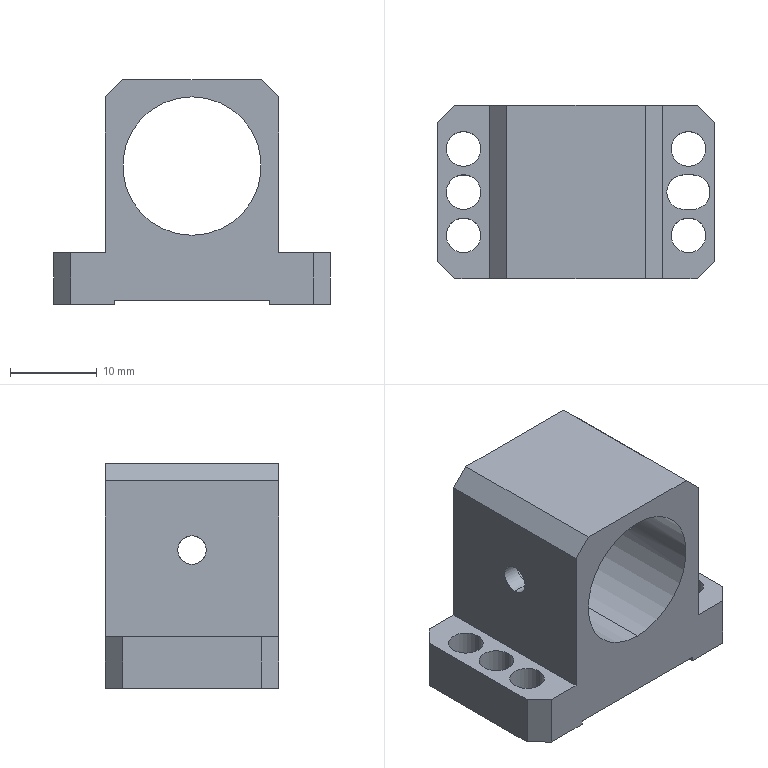Part | 1 solid | 41 faces | box 32 x 20 x 26 mm | volume 6999 mm3 | plane 22 | cylinder 19 | commonest cylinder face diameters 4 x13 3.3 x4 16 x2
STEP:
#1=CARTESIAN_POINT('',(-7.828,0.,-8.35));
#2=VERTEX_POINT('',#1);
#3=CARTESIAN_POINT('',(-7.828,0.,-11.65));
#4=VERTEX_POINT('',#3);
#5=CARTESIAN_POINT('',(-7.828,0.,-8.35));
#6=CARTESIAN_POINT('',(-7.828,-0.4372,-8.35));
#7=CARTESIAN_POINT('',(-7.915,-1.29,-8.708));
#8=CARTESIAN_POINT('',(-8.042,-1.83,-9.998));
#9=CARTESIAN_POINT('',(-7.915,-1.291,-11.293));
#10=CARTESIAN_POINT('',(-7.828,-0.4372,-11.65));
#11=CARTESIAN_POINT('',(-7.828,0.,-11.65));
#12=B_SPLINE_CURVE_WITH_KNOTS('',3,(#5,#6,#7,#8,#9,#10,#11),.UNSPECIFIED.,.F.,.F.,(4,1,1,1,4),(0.,0.001293,0.002586,0.003878,0.005171),.UNSPECIFIED.);
#13=EDGE_CURVE('',#2,#4,#12,.T.);
#14=ORIENTED_EDGE('',*,*,#13,.T.);
#15=CARTESIAN_POINT('',(-10.,0.,-11.65));
#16=VERTEX_POINT('',#15);
#17=CARTESIAN_POINT('',(-10.,0.,-11.65));
#18=DIRECTION('',(-1.,0.,0.));
#19=VECTOR('',#18,1000.);
#20=LINE('',#17,#19);
#21=EDGE_CURVE('',#4,#16,#20,.T.);
#22=ORIENTED_EDGE('',*,*,#21,.T.);
#23=CARTESIAN_POINT('',(-10.,0.,-8.35));
#24=VERTEX_POINT('',#23);
#25=CARTESIAN_POINT('',(-10.,0.,-10.));
#26=DIRECTION('',(-1.,0.,0.));
#27=DIRECTION('',(0.,0.,1.));
#28=AXIS2_PLACEMENT_3D('',#25,#26,#27);
#29=CIRCLE('',#28,1.65);
#30=EDGE_CURVE('',#16,#24,#29,.T.);
#31=ORIENTED_EDGE('',*,*,#30,.T.);
#32=CARTESIAN_POINT('',(-10.,0.,-8.35));
#33=DIRECTION('',(-1.,0.,0.));
#34=VECTOR('',#33,1000.);
#35=LINE('',#32,#34);
#36=EDGE_CURVE('',#2,#24,#35,.T.);
#37=ORIENTED_EDGE('',*,*,#36,.F.);
#38=EDGE_LOOP('',(#14,#22,#31,#37));
#39=FACE_BOUND('',#38,.T.);
#40=CARTESIAN_POINT('',(-10.,0.,-10.));
#41=DIRECTION('',(-1.,0.,0.));
#42=DIRECTION('',(0.,0.,-1.));
#43=AXIS2_PLACEMENT_3D('',#40,#41,#42);
#44=CYLINDRICAL_SURFACE('',#43,1.65);
#45=ADVANCED_FACE('',(#39),#44,.F.);
#46=CARTESIAN_POINT('',(7.828,0.,-11.65));
#47=VERTEX_POINT('',#46);
#48=CARTESIAN_POINT('',(7.828,0.,-8.35));
#49=VERTEX_POINT('',#48);
#50=CARTESIAN_POINT('',(7.828,0.,-11.65));
#51=CARTESIAN_POINT('',(7.828,-0.4372,-11.65));
#52=CARTESIAN_POINT('',(7.915,-1.29,-11.292));
#53=CARTESIAN_POINT('',(8.042,-1.83,-10.002));
#54=CARTESIAN_POINT('',(7.915,-1.291,-8.707));
#55=CARTESIAN_POINT('',(7.828,-0.4372,-8.35));
#56=CARTESIAN_POINT('',(7.828,0.,-8.35));
#57=B_SPLINE_CURVE_WITH_KNOTS('',3,(#50,#51,#52,#53,#54,#55,#56),.UNSPECIFIED.,.F.,.F.,(4,1,1,1,4),(0.,0.001293,0.002586,0.003878,0.005171),.UNSPECIFIED.);
#58=EDGE_CURVE('',#47,#49,#57,.T.);
#59=ORIENTED_EDGE('',*,*,#58,.T.);
#60=CARTESIAN_POINT('',(10.,0.,-8.35));
#61=VERTEX_POINT('',#60);
#62=CARTESIAN_POINT('',(10.,0.,-8.35));
#63=DIRECTION('',(1.,0.,0.));
#64=VECTOR('',#63,1000.);
#65=LINE('',#62,#64);
#66=EDGE_CURVE('',#49,#61,#65,.T.);
#67=ORIENTED_EDGE('',*,*,#66,.T.);
#68=CARTESIAN_POINT('',(10.,0.,-11.65));
#69=VERTEX_POINT('',#68);
#70=CARTESIAN_POINT('',(10.,0.,-10.));
#71=DIRECTION('',(1.,0.,0.));
#72=DIRECTION('',(0.,0.,-1.));
#73=AXIS2_PLACEMENT_3D('',#70,#71,#72);
#74=CIRCLE('',#73,1.65);
#75=EDGE_CURVE('',#61,#69,#74,.T.);
#76=ORIENTED_EDGE('',*,*,#75,.T.);
#77=CARTESIAN_POINT('',(10.,0.,-11.65));
#78=DIRECTION('',(1.,0.,0.));
#79=VECTOR('',#78,1000.);
#80=LINE('',#77,#79);
#81=EDGE_CURVE('',#47,#69,#80,.T.);
#82=ORIENTED_EDGE('',*,*,#81,.F.);
#83=EDGE_LOOP('',(#59,#67,#76,#82));
#84=FACE_BOUND('',#83,.T.);
#85=CARTESIAN_POINT('',(10.,0.,-10.));
#86=DIRECTION('',(1.,0.,0.));
#87=DIRECTION('',(0.,0.,1.));
#88=AXIS2_PLACEMENT_3D('',#85,#86,#87);
#89=CYLINDRICAL_SURFACE('',#88,1.65);
#90=ADVANCED_FACE('',(#84),#89,.F.);
#91=CARTESIAN_POINT('',(12.5,2.,-20.));
#92=VERTEX_POINT('',#91);
#93=CARTESIAN_POINT('',(10.5,0.,-20.));
#94=VERTEX_POINT('',#93);
#95=CARTESIAN_POINT('',(12.5,0.,-20.));
#96=DIRECTION('',(0.,0.,1.));
#97=DIRECTION('',(1.,0.,0.));
#98=AXIS2_PLACEMENT_3D('',#95,#96,#97);
#99=CIRCLE('',#98,2.);
#100=EDGE_CURVE('',#92,#94,#99,.T.);
#101=ORIENTED_EDGE('',*,*,#100,.T.);
#102=CARTESIAN_POINT('',(10.5,0.,-26.));
#103=VERTEX_POINT('',#102);
#104=CARTESIAN_POINT('',(10.5,0.,-16.));
#105=DIRECTION('',(0.,0.,-1.));
#106=VECTOR('',#105,1000.);
#107=LINE('',#104,#106);
#108=EDGE_CURVE('',#94,#103,#107,.T.);
#109=ORIENTED_EDGE('',*,*,#108,.T.);
#110=CARTESIAN_POINT('',(12.5,2.,-26.));
#111=VERTEX_POINT('',#110);
#112=CARTESIAN_POINT('',(12.5,0.,-26.));
#113=DIRECTION('',(0.,0.,-1.));
#114=DIRECTION('',(-1.,0.,0.));
#115=AXIS2_PLACEMENT_3D('',#112,#113,#114);
#116=CIRCLE('',#115,2.);
#117=EDGE_CURVE('',#103,#111,#116,.T.);
#118=ORIENTED_EDGE('',*,*,#117,.T.);
#119=CARTESIAN_POINT('',(12.5,2.,-16.));
#120=DIRECTION('',(0.,0.,-1.));
#121=VECTOR('',#120,1000.);
#122=LINE('',#119,#121);
#123=EDGE_CURVE('',#92,#111,#122,.T.);
#124=ORIENTED_EDGE('',*,*,#123,.F.);
#125=EDGE_LOOP('',(#101,#109,#118,#124));
#126=FACE_BOUND('',#125,.T.);
#127=CARTESIAN_POINT('',(12.5,0.,-16.));
#128=DIRECTION('',(0.,0.,-1.));
#129=DIRECTION('',(1.,0.,0.));
#130=AXIS2_PLACEMENT_3D('',#127,#128,#129);
#131=CYLINDRICAL_SURFACE('',#130,2.);
#132=ADVANCED_FACE('',(#126),#131,.F.);
#133=CARTESIAN_POINT('',(-15.,0.,-20.));
#134=VERTEX_POINT('',#133);
#135=CARTESIAN_POINT('',(-11.,0.,-20.));
#136=VERTEX_POINT('',#135);
#137=CARTESIAN_POINT('',(-13.,0.,-20.));
#138=DIRECTION('',(0.,0.,1.));
#139=DIRECTION('',(1.,0.,0.));
#140=AXIS2_PLACEMENT_3D('',#137,#138,#139);
#141=CIRCLE('',#140,2.);
#142=EDGE_CURVE('',#134,#136,#141,.T.);
#143=ORIENTED_EDGE('',*,*,#142,.T.);
#144=CARTESIAN_POINT('',(-11.,0.,-26.));
#145=VERTEX_POINT('',#144);
#146=CARTESIAN_POINT('',(-11.,0.,-16.));
#147=DIRECTION('',(0.,0.,-1.));
#148=VECTOR('',#147,1000.);
#149=LINE('',#146,#148);
#150=EDGE_CURVE('',#136,#145,#149,.T.);
#151=ORIENTED_EDGE('',*,*,#150,.T.);
#152=CARTESIAN_POINT('',(-15.,0.,-26.));
#153=VERTEX_POINT('',#152);
#154=CARTESIAN_POINT('',(-13.,0.,-26.));
#155=DIRECTION('',(0.,0.,-1.));
#156=DIRECTION('',(-1.,0.,0.));
#157=AXIS2_PLACEMENT_3D('',#154,#155,#156);
#158=CIRCLE('',#157,2.);
#159=EDGE_CURVE('',#145,#153,#158,.T.);
#160=ORIENTED_EDGE('',*,*,#159,.T.);
#161=CARTESIAN_POINT('',(-15.,0.,-16.));
#162=DIRECTION('',(0.,0.,-1.));
#163=VECTOR('',#162,1000.);
#164=LINE('',#161,#163);
#165=EDGE_CURVE('',#134,#153,#164,.T.);
#166=ORIENTED_EDGE('',*,*,#165,.F.);
#167=EDGE_LOOP('',(#143,#151,#160,#166));
#168=FACE_BOUND('',#167,.T.);
#169=CARTESIAN_POINT('',(-13.,0.,-16.));
#170=DIRECTION('',(0.,0.,-1.));
#171=DIRECTION('',(1.,0.,0.));
#172=AXIS2_PLACEMENT_3D('',#169,#170,#171);
#173=CYLINDRICAL_SURFACE('',#172,2.);
#174=ADVANCED_FACE('',(#168),#173,.F.);
#175=CARTESIAN_POINT('',(11.,-5.,-20.));
#176=VERTEX_POINT('',#175);
#177=CARTESIAN_POINT('',(15.,-5.,-20.));
#178=VERTEX_POINT('',#177);
#179=CARTESIAN_POINT('',(13.,-5.,-20.));
#180=DIRECTION('',(0.,0.,1.));
#181=DIRECTION('',(1.,0.,0.));
#182=AXIS2_PLACEMENT_3D('',#179,#180,#181);
#183=CIRCLE('',#182,2.);
#184=EDGE_CURVE('',#176,#178,#183,.T.);
#185=ORIENTED_EDGE('',*,*,#184,.T.);
#186=CARTESIAN_POINT('',(15.,-5.,-26.));
#187=VERTEX_POINT('',#186);
#188=CARTESIAN_POINT('',(15.,-5.,-6.));
#189=DIRECTION('',(0.,0.,-1.));
#190=VECTOR('',#189,1000.);
#191=LINE('',#188,#190);
#192=EDGE_CURVE('',#178,#187,#191,.T.);
#193=ORIENTED_EDGE('',*,*,#192,.T.);
#194=CARTESIAN_POINT('',(11.,-5.,-26.));
#195=VERTEX_POINT('',#194);
#196=CARTESIAN_POINT('',(13.,-5.,-26.));
#197=DIRECTION('',(0.,0.,-1.));
#198=DIRECTION('',(-1.,0.,0.));
#199=AXIS2_PLACEMENT_3D('',#196,#197,#198);
#200=CIRCLE('',#199,2.);
#201=EDGE_CURVE('',#187,#195,#200,.T.);
#202=ORIENTED_EDGE('',*,*,#201,.T.);
#203=CARTESIAN_POINT('',(11.,-5.,-6.));
#204=DIRECTION('',(0.,0.,-1.));
#205=VECTOR('',#204,1000.);
#206=LINE('',#203,#205);
#207=EDGE_CURVE('',#176,#195,#206,.T.);
#208=ORIENTED_EDGE('',*,*,#207,.F.);
#209=EDGE_LOOP('',(#185,#193,#202,#208));
#210=FACE_BOUND('',#209,.T.);
#211=CARTESIAN_POINT('',(13.,-5.,-6.));
#212=DIRECTION('',(0.,0.,-1.));
#213=DIRECTION('',(1.,0.,0.));
#214=AXIS2_PLACEMENT_3D('',#211,#212,#213);
#215=CYLINDRICAL_SURFACE('',#214,2.);
#216=ADVANCED_FACE('',(#210),#215,.F.);
#217=CARTESIAN_POINT('',(-15.,5.,-20.));
#218=VERTEX_POINT('',#217);
#219=CARTESIAN_POINT('',(-11.,5.,-20.));
#220=VERTEX_POINT('',#219);
#221=CARTESIAN_POINT('',(-13.,5.,-20.));
#222=DIRECTION('',(0.,0.,1.));
#223=DIRECTION('',(1.,0.,0.));
#224=AXIS2_PLACEMENT_3D('',#221,#222,#223);
#225=CIRCLE('',#224,2.);
#226=EDGE_CURVE('',#218,#220,#225,.T.);
#227=ORIENTED_EDGE('',*,*,#226,.T.);
#228=CARTESIAN_POINT('',(-11.,5.,-26.));
#229=VERTEX_POINT('',#228);
#230=CARTESIAN_POINT('',(-11.,5.,-6.));
#231=DIRECTION('',(0.,0.,-1.));
#232=VECTOR('',#231,1000.);
#233=LINE('',#230,#232);
#234=EDGE_CURVE('',#220,#229,#233,.T.);
#235=ORIENTED_EDGE('',*,*,#234,.T.);
#236=CARTESIAN_POINT('',(-15.,5.,-26.));
#237=VERTEX_POINT('',#236);
#238=CARTESIAN_POINT('',(-13.,5.,-26.));
#239=DIRECTION('',(0.,0.,-1.));
#240=DIRECTION('',(-1.,0.,0.));
#241=AXIS2_PLACEMENT_3D('',#238,#239,#240);
#242=CIRCLE('',#241,2.);
#243=EDGE_CURVE('',#229,#237,#242,.T.);
#244=ORIENTED_EDGE('',*,*,#243,.T.);
#245=CARTESIAN_POINT('',(-15.,5.,-6.));
#246=DIRECTION('',(0.,0.,-1.));
#247=VECTOR('',#246,1000.);
#248=LINE('',#245,#247);
#249=EDGE_CURVE('',#218,#237,#248,.T.);
#250=ORIENTED_EDGE('',*,*,#249,.F.);
#251=EDGE_LOOP('',(#227,#235,#244,#250));
#252=FACE_BOUND('',#251,.T.);
#253=CARTESIAN_POINT('',(-13.,5.,-6.));
#254=DIRECTION('',(0.,0.,-1.));
#255=DIRECTION('',(1.,0.,0.));
#256=AXIS2_PLACEMENT_3D('',#253,#254,#255);
#257=CYLINDRICAL_SURFACE('',#256,2.);
#258=ADVANCED_FACE('',(#252),#257,.F.);
#259=CARTESIAN_POINT('',(-15.,-5.,-20.));
#260=VERTEX_POINT('',#259);
#261=CARTESIAN_POINT('',(-11.,-5.,-20.));
#262=VERTEX_POINT('',#261);
#263=CARTESIAN_POINT('',(-13.,-5.,-20.));
#264=DIRECTION('',(0.,0.,1.));
#265=DIRECTION('',(1.,0.,0.));
#266=AXIS2_PLACEMENT_3D('',#263,#264,#265);
#267=CIRCLE('',#266,2.);
#268=EDGE_CURVE('',#260,#262,#267,.T.);
#269=ORIENTED_EDGE('',*,*,#268,.T.);
#270=CARTESIAN_POINT('',(-11.,-5.,-26.));
#271=VERTEX_POINT('',#270);
#272=CARTESIAN_POINT('',(-11.,-5.,-6.));
#273=DIRECTION('',(0.,0.,-1.));
#274=VECTOR('',#273,1000.);
#275=LINE('',#272,#274);
#276=EDGE_CURVE('',#262,#271,#275,.T.);
#277=ORIENTED_EDGE('',*,*,#276,.T.);
#278=CARTESIAN_POINT('',(-15.,-5.,-26.));
#279=VERTEX_POINT('',#278);
#280=CARTESIAN_POINT('',(-13.,-5.,-26.));
#281=DIRECTION('',(0.,0.,-1.));
#282=DIRECTION('',(-1.,0.,0.));
#283=AXIS2_PLACEMENT_3D('',#280,#281,#282);
#284=CIRCLE('',#283,2.);
#285=EDGE_CURVE('',#271,#279,#284,.T.);
#286=ORIENTED_EDGE('',*,*,#285,.T.);
#287=CARTESIAN_POINT('',(-15.,-5.,-6.));
#288=DIRECTION('',(0.,0.,-1.));
#289=VECTOR('',#288,1000.);
#290=LINE('',#287,#289);
#291=EDGE_CURVE('',#260,#279,#290,.T.);
#292=ORIENTED_EDGE('',*,*,#291,.F.);
#293=EDGE_LOOP('',(#269,#277,#286,#292));
#294=FACE_BOUND('',#293,.T.);
#295=CARTESIAN_POINT('',(-13.,-5.,-6.));
#296=DIRECTION('',(0.,0.,-1.));
#297=DIRECTION('',(1.,0.,0.));
#298=AXIS2_PLACEMENT_3D('',#295,#296,#297);
#299=CYLINDRICAL_SURFACE('',#298,2.);
#300=ADVANCED_FACE('',(#294),#299,.F.);
#301=CARTESIAN_POINT('',(11.,5.,-20.));
#302=VERTEX_POINT('',#301);
#303=CARTESIAN_POINT('',(15.,5.,-20.));
#304=VERTEX_POINT('',#303);
#305=CARTESIAN_POINT('',(13.,5.,-20.));
#306=DIRECTION('',(0.,0.,1.));
#307=DIRECTION('',(1.,0.,0.));
#308=AXIS2_PLACEMENT_3D('',#305,#306,#307);
#309=CIRCLE('',#308,2.);
#310=EDGE_CURVE('',#302,#304,#309,.T.);
#311=ORIENTED_EDGE('',*,*,#310,.T.);
#312=CARTESIAN_POINT('',(15.,5.,-26.));
#313=VERTEX_POINT('',#312);
#314=CARTESIAN_POINT('',(15.,5.,-6.));
#315=DIRECTION('',(0.,0.,-1.));
#316=VECTOR('',#315,1000.);
#317=LINE('',#314,#316);
#318=EDGE_CURVE('',#304,#313,#317,.T.);
#319=ORIENTED_EDGE('',*,*,#318,.T.);
#320=CARTESIAN_POINT('',(11.,5.,-26.));
#321=VERTEX_POINT('',#320);
#322=CARTESIAN_POINT('',(13.,5.,-26.));
#323=DIRECTION('',(0.,0.,-1.));
#324=DIRECTION('',(-1.,0.,0.));
#325=AXIS2_PLACEMENT_3D('',#322,#323,#324);
#326=CIRCLE('',#325,2.);
#327=EDGE_CURVE('',#313,#321,#326,.T.);
#328=ORIENTED_EDGE('',*,*,#327,.T.);
#329=CARTESIAN_POINT('',(11.,5.,-6.));
#330=DIRECTION('',(0.,0.,-1.));
#331=VECTOR('',#330,1000.);
#332=LINE('',#329,#331);
#333=EDGE_CURVE('',#302,#321,#332,.T.);
#334=ORIENTED_EDGE('',*,*,#333,.F.);
#335=EDGE_LOOP('',(#311,#319,#328,#334));
#336=FACE_BOUND('',#335,.T.);
#337=CARTESIAN_POINT('',(13.,5.,-6.));
#338=DIRECTION('',(0.,0.,-1.));
#339=DIRECTION('',(1.,0.,0.));
#340=AXIS2_PLACEMENT_3D('',#337,#338,#339);
#341=CYLINDRICAL_SURFACE('',#340,2.);
#342=ADVANCED_FACE('',(#336),#341,.F.);
#343=ORIENTED_EDGE('',*,*,#13,.F.);
#344=CARTESIAN_POINT('',(-7.828,0.,-11.65));
#345=CARTESIAN_POINT('',(-7.828,0.4372,-11.65));
#346=CARTESIAN_POINT('',(-7.915,1.29,-11.292));
#347=CARTESIAN_POINT('',(-8.042,1.83,-10.002));
#348=CARTESIAN_POINT('',(-7.915,1.291,-8.707));
#349=CARTESIAN_POINT('',(-7.828,0.4372,-8.35));
#350=CARTESIAN_POINT('',(-7.828,0.,-8.35));
#351=B_SPLINE_CURVE_WITH_KNOTS('',3,(#344,#345,#346,#347,#348,#349,#350),.UNSPECIFIED.,.F.,.F.,(4,1,1,1,4),(0.,0.001293,0.002586,0.003878,0.005171),.UNSPECIFIED.);
#352=EDGE_CURVE('',#4,#2,#351,.T.);
#353=ORIENTED_EDGE('',*,*,#352,.F.);
#354=EDGE_LOOP('',(#343,#353));
#355=FACE_BOUND('',#354,.T.);
#356=CARTESIAN_POINT('',(0.,10.,-18.));
#357=VERTEX_POINT('',#356);
#358=CARTESIAN_POINT('',(0.,10.,-2.));
#359=VERTEX_POINT('',#358);
#360=CARTESIAN_POINT('',(0.,10.,-10.));
#361=DIRECTION('',(0.,1.,0.));
#362=DIRECTION('',(0.,0.,1.));
#363=AXIS2_PLACEMENT_3D('',#360,#361,#362);
#364=CIRCLE('',#363,8.);
#365=EDGE_CURVE('',#357,#359,#364,.T.);
#366=ORIENTED_EDGE('',*,*,#365,.T.);
#367=CARTESIAN_POINT('',(0.,-10.,-2.));
#368=VERTEX_POINT('',#367);
#369=CARTESIAN_POINT('',(0.,10.,-2.));
#370=DIRECTION('',(0.,-1.,0.));
#371=VECTOR('',#370,1000.);
#372=LINE('',#369,#371);
#373=EDGE_CURVE('',#359,#368,#372,.T.);
#374=ORIENTED_EDGE('',*,*,#373,.T.);
#375=CARTESIAN_POINT('',(0.,-10.,-18.));
#376=VERTEX_POINT('',#375);
#377=CARTESIAN_POINT('',(0.,-10.,-10.));
#378=DIRECTION('',(0.,1.,0.));
#379=DIRECTION('',(0.,0.,1.));
#380=AXIS2_PLACEMENT_3D('',#377,#378,#379);
#381=CIRCLE('',#380,8.);
#382=EDGE_CURVE('',#376,#368,#381,.T.);
#383=ORIENTED_EDGE('',*,*,#382,.F.);
#384=CARTESIAN_POINT('',(0.,10.,-18.));
#385=DIRECTION('',(0.,-1.,0.));
#386=VECTOR('',#385,1000.);
#387=LINE('',#384,#386);
#388=EDGE_CURVE('',#357,#376,#387,.T.);
#389=ORIENTED_EDGE('',*,*,#388,.F.);
#390=EDGE_LOOP('',(#366,#374,#383,#389));
#391=FACE_BOUND('',#390,.T.);
#392=CARTESIAN_POINT('',(0.,10.,-10.));
#393=DIRECTION('',(0.,-1.,0.));
#394=DIRECTION('',(0.,0.,1.));
#395=AXIS2_PLACEMENT_3D('',#392,#393,#394);
#396=CYLINDRICAL_SURFACE('',#395,8.);
#397=ADVANCED_FACE('',(#355,#391),#396,.F.);
#398=CARTESIAN_POINT('',(13.,5.,-26.));
#399=DIRECTION('',(0.,0.,-1.));
#400=DIRECTION('',(-1.,0.,0.));
#401=AXIS2_PLACEMENT_3D('',#398,#399,#400);
#402=CIRCLE('',#401,2.);
#403=EDGE_CURVE('',#321,#313,#402,.T.);
#404=ORIENTED_EDGE('',*,*,#403,.F.);
#405=ORIENTED_EDGE('',*,*,#327,.F.);
#406=EDGE_LOOP('',(#404,#405));
#407=FACE_BOUND('',#406,.T.);
#408=CARTESIAN_POINT('',(13.,-5.,-26.));
#409=DIRECTION('',(0.,0.,-1.));
#410=DIRECTION('',(-1.,0.,0.));
#411=AXIS2_PLACEMENT_3D('',#408,#409,#410);
#412=CIRCLE('',#411,2.);
#413=EDGE_CURVE('',#195,#187,#412,.T.);
#414=ORIENTED_EDGE('',*,*,#413,.F.);
#415=ORIENTED_EDGE('',*,*,#201,.F.);
#416=EDGE_LOOP('',(#414,#415));
#417=FACE_BOUND('',#416,.T.);
#418=CARTESIAN_POINT('',(13.5,-2.,-26.));
#419=VERTEX_POINT('',#418);
#420=CARTESIAN_POINT('',(12.5,-2.,-26.));
#421=VERTEX_POINT('',#420);
#422=CARTESIAN_POINT('',(12.5,-2.,-26.));
#423=DIRECTION('',(-1.,0.,0.));
#424=VECTOR('',#423,1000.);
#425=LINE('',#422,#424);
#426=EDGE_CURVE('',#419,#421,#425,.T.);
#427=ORIENTED_EDGE('',*,*,#426,.F.);
#428=CARTESIAN_POINT('',(13.5,2.,-26.));
#429=VERTEX_POINT('',#428);
#430=CARTESIAN_POINT('',(13.5,0.,-26.));
#431=DIRECTION('',(0.,0.,-1.));
#432=DIRECTION('',(-1.,0.,0.));
#433=AXIS2_PLACEMENT_3D('',#430,#431,#432);
#434=CIRCLE('',#433,2.);
#435=EDGE_CURVE('',#429,#419,#434,.T.);
#436=ORIENTED_EDGE('',*,*,#435,.F.);
#437=CARTESIAN_POINT('',(12.5,2.,-26.));
#438=DIRECTION('',(1.,0.,0.));
#439=VECTOR('',#438,1000.);
#440=LINE('',#437,#439);
#441=EDGE_CURVE('',#111,#429,#440,.T.);
#442=ORIENTED_EDGE('',*,*,#441,.F.);
#443=ORIENTED_EDGE('',*,*,#117,.F.);
#444=CARTESIAN_POINT('',(12.5,0.,-26.));
#445=DIRECTION('',(0.,0.,-1.));
#446=DIRECTION('',(-1.,0.,0.));
#447=AXIS2_PLACEMENT_3D('',#444,#445,#446);
#448=CIRCLE('',#447,2.);
#449=EDGE_CURVE('',#421,#103,#448,.T.);
#450=ORIENTED_EDGE('',*,*,#449,.F.);
#451=EDGE_LOOP('',(#427,#436,#442,#443,#450));
#452=FACE_BOUND('',#451,.T.);
#453=CARTESIAN_POINT('',(14.,-10.,-26.));
#454=VERTEX_POINT('',#453);
#455=CARTESIAN_POINT('',(9.,-10.,-26.));
#456=VERTEX_POINT('',#455);
#457=CARTESIAN_POINT('',(10.,-10.,-26.));
#458=DIRECTION('',(-1.,0.,0.));
#459=VECTOR('',#458,1000.);
#460=LINE('',#457,#459);
#461=EDGE_CURVE('',#454,#456,#460,.T.);
#462=ORIENTED_EDGE('',*,*,#461,.T.);
#463=CARTESIAN_POINT('',(9.,10.,-26.));
#464=VERTEX_POINT('',#463);
#465=CARTESIAN_POINT('',(9.,10.,-26.));
#466=DIRECTION('',(0.,-1.,0.));
#467=VECTOR('',#466,1000.);
#468=LINE('',#465,#467);
#469=EDGE_CURVE('',#464,#456,#468,.T.);
#470=ORIENTED_EDGE('',*,*,#469,.F.);
#471=CARTESIAN_POINT('',(14.,10.,-26.));
#472=VERTEX_POINT('',#471);
#473=CARTESIAN_POINT('',(10.,10.,-26.));
#474=DIRECTION('',(-1.,0.,0.));
#475=VECTOR('',#474,1000.);
#476=LINE('',#473,#475);
#477=EDGE_CURVE('',#472,#464,#476,.T.);
#478=ORIENTED_EDGE('',*,*,#477,.F.);
#479=CARTESIAN_POINT('',(16.,8.,-26.));
#480=VERTEX_POINT('',#479);
#481=CARTESIAN_POINT('',(16.,8.,-26.));
#482=DIRECTION('',(0.7071,-0.7071,0.));
#483=VECTOR('',#482,1000.);
#484=LINE('',#481,#483);
#485=EDGE_CURVE('',#472,#480,#484,.T.);
#486=ORIENTED_EDGE('',*,*,#485,.T.);
#487=CARTESIAN_POINT('',(16.,-8.,-26.));
#488=VERTEX_POINT('',#487);
#489=CARTESIAN_POINT('',(16.,10.,-26.));
#490=DIRECTION('',(0.,-1.,0.));
#491=VECTOR('',#490,1000.);
#492=LINE('',#489,#491);
#493=EDGE_CURVE('',#480,#488,#492,.T.);
#494=ORIENTED_EDGE('',*,*,#493,.T.);
#495=CARTESIAN_POINT('',(14.,-10.,-26.));
#496=DIRECTION('',(-0.7071,-0.7071,0.));
#497=VECTOR('',#496,1000.);
#498=LINE('',#495,#497);
#499=EDGE_CURVE('',#488,#454,#498,.T.);
#500=ORIENTED_EDGE('',*,*,#499,.T.);
#501=EDGE_LOOP('',(#462,#470,#478,#486,#494,#500));
#502=FACE_BOUND('',#501,.T.);
#503=CARTESIAN_POINT('',(10.,10.,-26.));
#504=DIRECTION('',(0.,0.,1.));
#505=DIRECTION('',(-1.,0.,0.));
#506=AXIS2_PLACEMENT_3D('',#503,#504,#505);
#507=PLANE('',#506);
#508=ADVANCED_FACE('',(#407,#417,#452,#502),#507,.F.);
#509=CARTESIAN_POINT('',(9.,10.,-25.5));
#510=VERTEX_POINT('',#509);
#511=CARTESIAN_POINT('',(9.,10.,-25.5));
#512=DIRECTION('',(0.,0.,-1.));
#513=VECTOR('',#512,1000.);
#514=LINE('',#511,#513);
#515=EDGE_CURVE('',#510,#464,#514,.T.);
#516=ORIENTED_EDGE('',*,*,#515,.F.);
#517=CARTESIAN_POINT('',(-9.,10.,-25.5));
#518=VERTEX_POINT('',#517);
#519=CARTESIAN_POINT('',(9.,10.,-25.5));
#520=DIRECTION('',(1.,0.,0.));
#521=VECTOR('',#520,1000.);
#522=LINE('',#519,#521);
#523=EDGE_CURVE('',#518,#510,#522,.T.);
#524=ORIENTED_EDGE('',*,*,#523,.F.);
#525=CARTESIAN_POINT('',(-9.,10.,-26.));
#526=VERTEX_POINT('',#525);
#527=CARTESIAN_POINT('',(-9.,10.,-25.5));
#528=DIRECTION('',(0.,0.,-1.));
#529=VECTOR('',#528,1000.);
#530=LINE('',#527,#529);
#531=EDGE_CURVE('',#518,#526,#530,.T.);
#532=ORIENTED_EDGE('',*,*,#531,.T.);
#533=CARTESIAN_POINT('',(-14.,10.,-26.));
#534=VERTEX_POINT('',#533);
#535=CARTESIAN_POINT('',(10.,10.,-26.));
#536=DIRECTION('',(-1.,0.,0.));
#537=VECTOR('',#536,1000.);
#538=LINE('',#535,#537);
#539=EDGE_CURVE('',#526,#534,#538,.T.);
#540=ORIENTED_EDGE('',*,*,#539,.T.);
#541=CARTESIAN_POINT('',(-14.,10.,-20.));
#542=VERTEX_POINT('',#541);
#543=CARTESIAN_POINT('',(-14.,10.,-13.));
#544=DIRECTION('',(0.,0.,1.));
#545=VECTOR('',#544,1000.);
#546=LINE('',#543,#545);
#547=EDGE_CURVE('',#534,#542,#546,.T.);
#548=ORIENTED_EDGE('',*,*,#547,.T.);
#549=CARTESIAN_POINT('',(-10.,10.,-20.));
#550=VERTEX_POINT('',#549);
#551=CARTESIAN_POINT('',(-16.,10.,-20.));
#552=DIRECTION('',(-1.,0.,0.));
#553=VECTOR('',#552,1000.);
#554=LINE('',#551,#553);
#555=EDGE_CURVE('',#550,#542,#554,.T.);
#556=ORIENTED_EDGE('',*,*,#555,.F.);
#557=CARTESIAN_POINT('',(-10.,10.,-2.));
#558=VERTEX_POINT('',#557);
#559=CARTESIAN_POINT('',(-10.,10.,0.));
#560=DIRECTION('',(0.,0.,1.));
#561=VECTOR('',#560,1000.);
#562=LINE('',#559,#561);
#563=EDGE_CURVE('',#550,#558,#562,.T.);
#564=ORIENTED_EDGE('',*,*,#563,.T.);
#565=CARTESIAN_POINT('',(-8.,10.,0.));
#566=VERTEX_POINT('',#565);
#567=CARTESIAN_POINT('',(-10.5,10.,-2.5));
#568=DIRECTION('',(0.7071,0.,0.7071));
#569=VECTOR('',#568,1000.);
#570=LINE('',#567,#569);
#571=EDGE_CURVE('',#558,#566,#570,.T.);
#572=ORIENTED_EDGE('',*,*,#571,.T.);
#573=CARTESIAN_POINT('',(8.,10.,0.));
#574=VERTEX_POINT('',#573);
#575=CARTESIAN_POINT('',(10.,10.,0.));
#576=DIRECTION('',(1.,0.,0.));
#577=VECTOR('',#576,1000.);
#578=LINE('',#575,#577);
#579=EDGE_CURVE('',#566,#574,#578,.T.);
#580=ORIENTED_EDGE('',*,*,#579,.T.);
#581=CARTESIAN_POINT('',(10.,10.,-2.));
#582=VERTEX_POINT('',#581);
#583=CARTESIAN_POINT('',(10.5,10.,-2.5));
#584=DIRECTION('',(0.7071,0.,-0.7071));
#585=VECTOR('',#584,1000.);
#586=LINE('',#583,#585);
#587=EDGE_CURVE('',#574,#582,#586,.T.);
#588=ORIENTED_EDGE('',*,*,#587,.T.);
#589=CARTESIAN_POINT('',(10.,10.,-20.));
#590=VERTEX_POINT('',#589);
#591=CARTESIAN_POINT('',(10.,10.,0.));
#592=DIRECTION('',(0.,0.,-1.));
#593=VECTOR('',#592,1000.);
#594=LINE('',#591,#593);
#595=EDGE_CURVE('',#582,#590,#594,.T.);
#596=ORIENTED_EDGE('',*,*,#595,.T.);
#597=CARTESIAN_POINT('',(14.,10.,-20.));
#598=VERTEX_POINT('',#597);
#599=CARTESIAN_POINT('',(-16.,10.,-20.));
#600=DIRECTION('',(-1.,0.,0.));
#601=VECTOR('',#600,1000.);
#602=LINE('',#599,#601);
#603=EDGE_CURVE('',#598,#590,#602,.T.);
#604=ORIENTED_EDGE('',*,*,#603,.F.);
#605=CARTESIAN_POINT('',(14.,10.,-13.));
#606=DIRECTION('',(0.,0.,-1.));
#607=VECTOR('',#606,1000.);
#608=LINE('',#605,#607);
#609=EDGE_CURVE('',#598,#472,#608,.T.);
#610=ORIENTED_EDGE('',*,*,#609,.T.);
#611=ORIENTED_EDGE('',*,*,#477,.T.);
#612=EDGE_LOOP('',(#516,#524,#532,#540,#548,#556,#564,#572,#580,#588,#596,#604,#610,#611));
#613=FACE_BOUND('',#612,.T.);
#614=ORIENTED_EDGE('',*,*,#365,.F.);
#615=CARTESIAN_POINT('',(0.,10.,-10.));
#616=DIRECTION('',(0.,1.,0.));
#617=DIRECTION('',(0.,0.,1.));
#618=AXIS2_PLACEMENT_3D('',#615,#616,#617);
#619=CIRCLE('',#618,8.);
#620=EDGE_CURVE('',#359,#357,#619,.T.);
#621=ORIENTED_EDGE('',*,*,#620,.F.);
#622=EDGE_LOOP('',(#614,#621));
#623=FACE_BOUND('',#622,.T.);
#624=CARTESIAN_POINT('',(0.,10.,-13.));
#625=DIRECTION('',(0.,1.,0.));
#626=DIRECTION('',(0.,0.,-1.));
#627=AXIS2_PLACEMENT_3D('',#624,#625,#626);
#628=PLANE('',#627);
#629=ADVANCED_FACE('',(#613,#623),#628,.T.);
#630=CARTESIAN_POINT('',(9.,-10.,-25.5));
#631=VERTEX_POINT('',#630);
#632=CARTESIAN_POINT('',(-9.,-10.,-25.5));
#633=VERTEX_POINT('',#632);
#634=CARTESIAN_POINT('',(9.,-10.,-25.5));
#635=DIRECTION('',(-1.,0.,0.));
#636=VECTOR('',#635,1000.);
#637=LINE('',#634,#636);
#638=EDGE_CURVE('',#631,#633,#637,.T.);
#639=ORIENTED_EDGE('',*,*,#638,.F.);
#640=CARTESIAN_POINT('',(9.,-10.,-25.5));
#641=DIRECTION('',(0.,0.,-1.));
#642=VECTOR('',#641,1000.);
#643=LINE('',#640,#642);
#644=EDGE_CURVE('',#631,#456,#643,.T.);
#645=ORIENTED_EDGE('',*,*,#644,.T.);
#646=ORIENTED_EDGE('',*,*,#461,.F.);
#647=CARTESIAN_POINT('',(14.,-10.,-20.));
#648=VERTEX_POINT('',#647);
#649=CARTESIAN_POINT('',(14.,-10.,-20.));
#650=DIRECTION('',(0.,0.,1.));
#651=VECTOR('',#650,1000.);
#652=LINE('',#649,#651);
#653=EDGE_CURVE('',#454,#648,#652,.T.);
#654=ORIENTED_EDGE('',*,*,#653,.T.);
#655=CARTESIAN_POINT('',(10.,-10.,-20.));
#656=VERTEX_POINT('',#655);
#657=CARTESIAN_POINT('',(-16.,-10.,-20.));
#658=DIRECTION('',(-1.,0.,0.));
#659=VECTOR('',#658,1000.);
#660=LINE('',#657,#659);
#661=EDGE_CURVE('',#648,#656,#660,.T.);
#662=ORIENTED_EDGE('',*,*,#661,.T.);
#663=CARTESIAN_POINT('',(10.,-10.,-2.));
#664=VERTEX_POINT('',#663);
#665=CARTESIAN_POINT('',(10.,-10.,0.));
#666=DIRECTION('',(0.,0.,-1.));
#667=VECTOR('',#666,1000.);
#668=LINE('',#665,#667);
#669=EDGE_CURVE('',#664,#656,#668,.T.);
#670=ORIENTED_EDGE('',*,*,#669,.F.);
#671=CARTESIAN_POINT('',(8.,-10.,0.));
#672=VERTEX_POINT('',#671);
#673=CARTESIAN_POINT('',(10.,-10.,-2.));
#674=DIRECTION('',(-0.7071,0.,0.7071));
#675=VECTOR('',#674,1000.);
#676=LINE('',#673,#675);
#677=EDGE_CURVE('',#664,#672,#676,.T.);
#678=ORIENTED_EDGE('',*,*,#677,.T.);
#679=CARTESIAN_POINT('',(-8.,-10.,0.));
#680=VERTEX_POINT('',#679);
#681=CARTESIAN_POINT('',(10.,-10.,0.));
#682=DIRECTION('',(1.,0.,0.));
#683=VECTOR('',#682,1000.);
#684=LINE('',#681,#683);
#685=EDGE_CURVE('',#680,#672,#684,.T.);
#686=ORIENTED_EDGE('',*,*,#685,.F.);
#687=CARTESIAN_POINT('',(-10.,-10.,-2.));
#688=VERTEX_POINT('',#687);
#689=CARTESIAN_POINT('',(-8.,-10.,0.));
#690=DIRECTION('',(-0.7071,0.,-0.7071));
#691=VECTOR('',#690,1000.);
#692=LINE('',#689,#691);
#693=EDGE_CURVE('',#680,#688,#692,.T.);
#694=ORIENTED_EDGE('',*,*,#693,.T.);
#695=CARTESIAN_POINT('',(-10.,-10.,-20.));
#696=VERTEX_POINT('',#695);
#697=CARTESIAN_POINT('',(-10.,-10.,0.));
#698=DIRECTION('',(0.,0.,1.));
#699=VECTOR('',#698,1000.);
#700=LINE('',#697,#699);
#701=EDGE_CURVE('',#696,#688,#700,.T.);
#702=ORIENTED_EDGE('',*,*,#701,.F.);
#703=CARTESIAN_POINT('',(-14.,-10.,-20.));
#704=VERTEX_POINT('',#703);
#705=CARTESIAN_POINT('',(-16.,-10.,-20.));
#706=DIRECTION('',(-1.,0.,0.));
#707=VECTOR('',#706,1000.);
#708=LINE('',#705,#707);
#709=EDGE_CURVE('',#696,#704,#708,.T.);
#710=ORIENTED_EDGE('',*,*,#709,.T.);
#711=CARTESIAN_POINT('',(-14.,-10.,-26.));
#712=VERTEX_POINT('',#711);
#713=CARTESIAN_POINT('',(-14.,-10.,-26.));
#714=DIRECTION('',(0.,0.,-1.));
#715=VECTOR('',#714,1000.);
#716=LINE('',#713,#715);
#717=EDGE_CURVE('',#704,#712,#716,.T.);
#718=ORIENTED_EDGE('',*,*,#717,.T.);
#719=CARTESIAN_POINT('',(-9.,-10.,-26.));
#720=VERTEX_POINT('',#719);
#721=CARTESIAN_POINT('',(10.,-10.,-26.));
#722=DIRECTION('',(-1.,0.,0.));
#723=VECTOR('',#722,1000.);
#724=LINE('',#721,#723);
#725=EDGE_CURVE('',#720,#712,#724,.T.);
#726=ORIENTED_EDGE('',*,*,#725,.F.);
#727=CARTESIAN_POINT('',(-9.,-10.,-25.5));
#728=DIRECTION('',(0.,0.,-1.));
#729=VECTOR('',#728,1000.);
#730=LINE('',#727,#729);
#731=EDGE_CURVE('',#633,#720,#730,.T.);
#732=ORIENTED_EDGE('',*,*,#731,.F.);
#733=EDGE_LOOP('',(#639,#645,#646,#654,#662,#670,#678,#686,#694,#702,#710,#718,#726,#732));
#734=FACE_BOUND('',#733,.T.);
#735=ORIENTED_EDGE('',*,*,#382,.T.);
#736=CARTESIAN_POINT('',(0.,-10.,-10.));
#737=DIRECTION('',(0.,1.,0.));
#738=DIRECTION('',(0.,0.,1.));
#739=AXIS2_PLACEMENT_3D('',#736,#737,#738);
#740=CIRCLE('',#739,8.);
#741=EDGE_CURVE('',#368,#376,#740,.T.);
#742=ORIENTED_EDGE('',*,*,#741,.T.);
#743=EDGE_LOOP('',(#735,#742));
#744=FACE_BOUND('',#743,.T.);
#745=CARTESIAN_POINT('',(0.,-10.,-13.));
#746=DIRECTION('',(0.,1.,0.));
#747=DIRECTION('',(0.,0.,-1.));
#748=AXIS2_PLACEMENT_3D('',#745,#746,#747);
#749=PLANE('',#748);
#750=ADVANCED_FACE('',(#734,#744),#749,.F.);
#751=CARTESIAN_POINT('',(-10.,0.,-10.));
#752=DIRECTION('',(-1.,0.,0.));
#753=DIRECTION('',(0.,0.,1.));
#754=AXIS2_PLACEMENT_3D('',#751,#752,#753);
#755=CIRCLE('',#754,1.65);
#756=EDGE_CURVE('',#24,#16,#755,.T.);
#757=ORIENTED_EDGE('',*,*,#756,.F.);
#758=ORIENTED_EDGE('',*,*,#30,.F.);
#759=EDGE_LOOP('',(#757,#758));
#760=FACE_BOUND('',#759,.T.);
#761=ORIENTED_EDGE('',*,*,#701,.T.);
#762=CARTESIAN_POINT('',(-10.,10.,-2.));
#763=DIRECTION('',(0.,1.,0.));
#764=VECTOR('',#763,1000.);
#765=LINE('',#762,#764);
#766=EDGE_CURVE('',#688,#558,#765,.T.);
#767=ORIENTED_EDGE('',*,*,#766,.T.);
#768=ORIENTED_EDGE('',*,*,#563,.F.);
#769=CARTESIAN_POINT('',(-10.,10.,-20.));
#770=DIRECTION('',(0.,-1.,0.));
#771=VECTOR('',#770,1000.);
#772=LINE('',#769,#771);
#773=EDGE_CURVE('',#550,#696,#772,.T.);
#774=ORIENTED_EDGE('',*,*,#773,.T.);
#775=EDGE_LOOP('',(#761,#767,#768,#774));
#776=FACE_BOUND('',#775,.T.);
#777=CARTESIAN_POINT('',(-10.,10.,0.));
#778=DIRECTION('',(1.,0.,0.));
#779=DIRECTION('',(0.,0.,1.));
#780=AXIS2_PLACEMENT_3D('',#777,#778,#779);
#781=PLANE('',#780);
#782=ADVANCED_FACE('',(#760,#776),#781,.F.);
#783=ORIENTED_EDGE('',*,*,#579,.F.);
#784=CARTESIAN_POINT('',(-8.,10.,0.));
#785=DIRECTION('',(0.,-1.,0.));
#786=VECTOR('',#785,1000.);
#787=LINE('',#784,#786);
#788=EDGE_CURVE('',#566,#680,#787,.T.);
#789=ORIENTED_EDGE('',*,*,#788,.T.);
#790=ORIENTED_EDGE('',*,*,#685,.T.);
#791=CARTESIAN_POINT('',(8.,10.,0.));
#792=DIRECTION('',(0.,1.,0.));
#793=VECTOR('',#792,1000.);
#794=LINE('',#791,#793);
#795=EDGE_CURVE('',#672,#574,#794,.T.);
#796=ORIENTED_EDGE('',*,*,#795,.T.);
#797=EDGE_LOOP('',(#783,#789,#790,#796));
#798=FACE_BOUND('',#797,.T.);
#799=CARTESIAN_POINT('',(10.,10.,0.));
#800=DIRECTION('',(0.,0.,-1.));
#801=DIRECTION('',(1.,0.,0.));
#802=AXIS2_PLACEMENT_3D('',#799,#800,#801);
#803=PLANE('',#802);
#804=ADVANCED_FACE('',(#798),#803,.F.);
#805=CARTESIAN_POINT('',(10.,0.,-10.));
#806=DIRECTION('',(1.,0.,0.));
#807=DIRECTION('',(0.,0.,-1.));
#808=AXIS2_PLACEMENT_3D('',#805,#806,#807);
#809=CIRCLE('',#808,1.65);
#810=EDGE_CURVE('',#69,#61,#809,.T.);
#811=ORIENTED_EDGE('',*,*,#810,.F.);
#812=ORIENTED_EDGE('',*,*,#75,.F.);
#813=EDGE_LOOP('',(#811,#812));
#814=FACE_BOUND('',#813,.T.);
#815=ORIENTED_EDGE('',*,*,#595,.F.);
#816=CARTESIAN_POINT('',(10.,10.,-2.));
#817=DIRECTION('',(0.,-1.,0.));
#818=VECTOR('',#817,1000.);
#819=LINE('',#816,#818);
#820=EDGE_CURVE('',#582,#664,#819,.T.);
#821=ORIENTED_EDGE('',*,*,#820,.T.);
#822=ORIENTED_EDGE('',*,*,#669,.T.);
#823=CARTESIAN_POINT('',(10.,10.,-20.));
#824=DIRECTION('',(0.,1.,0.));
#825=VECTOR('',#824,1000.);
#826=LINE('',#823,#825);
#827=EDGE_CURVE('',#656,#590,#826,.T.);
#828=ORIENTED_EDGE('',*,*,#827,.T.);
#829=EDGE_LOOP('',(#815,#821,#822,#828));
#830=FACE_BOUND('',#829,.T.);
#831=CARTESIAN_POINT('',(10.,10.,0.));
#832=DIRECTION('',(-1.,0.,0.));
#833=DIRECTION('',(0.,0.,-1.));
#834=AXIS2_PLACEMENT_3D('',#831,#832,#833);
#835=PLANE('',#834);
#836=ADVANCED_FACE('',(#814,#830),#835,.F.);
#837=CARTESIAN_POINT('',(-13.,0.,-26.));
#838=DIRECTION('',(0.,0.,-1.));
#839=DIRECTION('',(-1.,0.,0.));
#840=AXIS2_PLACEMENT_3D('',#837,#838,#839);
#841=CIRCLE('',#840,2.);
#842=EDGE_CURVE('',#153,#145,#841,.T.);
#843=ORIENTED_EDGE('',*,*,#842,.F.);
#844=ORIENTED_EDGE('',*,*,#159,.F.);
#845=EDGE_LOOP('',(#843,#844));
#846=FACE_BOUND('',#845,.T.);
#847=CARTESIAN_POINT('',(-13.,5.,-26.));
#848=DIRECTION('',(0.,0.,-1.));
#849=DIRECTION('',(-1.,0.,0.));
#850=AXIS2_PLACEMENT_3D('',#847,#848,#849);
#851=CIRCLE('',#850,2.);
#852=EDGE_CURVE('',#237,#229,#851,.T.);
#853=ORIENTED_EDGE('',*,*,#852,.F.);
#854=ORIENTED_EDGE('',*,*,#243,.F.);
#855=EDGE_LOOP('',(#853,#854));
#856=FACE_BOUND('',#855,.T.);
#857=CARTESIAN_POINT('',(-13.,-5.,-26.));
#858=DIRECTION('',(0.,0.,-1.));
#859=DIRECTION('',(-1.,0.,0.));
#860=AXIS2_PLACEMENT_3D('',#857,#858,#859);
#861=CIRCLE('',#860,2.);
#862=EDGE_CURVE('',#279,#271,#861,.T.);
#863=ORIENTED_EDGE('',*,*,#862,.F.);
#864=ORIENTED_EDGE('',*,*,#285,.F.);
#865=EDGE_LOOP('',(#863,#864));
#866=FACE_BOUND('',#865,.T.);
#867=ORIENTED_EDGE('',*,*,#539,.F.);
#868=CARTESIAN_POINT('',(-9.,10.,-26.));
#869=DIRECTION('',(0.,1.,0.));
#870=VECTOR('',#869,1000.);
#871=LINE('',#868,#870);
#872=EDGE_CURVE('',#720,#526,#871,.T.);
#873=ORIENTED_EDGE('',*,*,#872,.F.);
#874=ORIENTED_EDGE('',*,*,#725,.T.);
#875=CARTESIAN_POINT('',(-16.,-8.,-26.));
#876=VERTEX_POINT('',#875);
#877=CARTESIAN_POINT('',(-14.,-10.,-26.));
#878=DIRECTION('',(-0.7071,0.7071,0.));
#879=VECTOR('',#878,1000.);
#880=LINE('',#877,#879);
#881=EDGE_CURVE('',#712,#876,#880,.T.);
#882=ORIENTED_EDGE('',*,*,#881,.T.);
#883=CARTESIAN_POINT('',(-16.,8.,-26.));
#884=VERTEX_POINT('',#883);
#885=CARTESIAN_POINT('',(-16.,10.,-26.));
#886=DIRECTION('',(0.,-1.,0.));
#887=VECTOR('',#886,1000.);
#888=LINE('',#885,#887);
#889=EDGE_CURVE('',#884,#876,#888,.T.);
#890=ORIENTED_EDGE('',*,*,#889,.F.);
#891=CARTESIAN_POINT('',(-16.,8.,-26.));
#892=DIRECTION('',(0.7071,0.7071,0.));
#893=VECTOR('',#892,1000.);
#894=LINE('',#891,#893);
#895=EDGE_CURVE('',#884,#534,#894,.T.);
#896=ORIENTED_EDGE('',*,*,#895,.T.);
#897=EDGE_LOOP('',(#867,#873,#874,#882,#890,#896));
#898=FACE_BOUND('',#897,.T.);
#899=CARTESIAN_POINT('',(10.,10.,-26.));
#900=DIRECTION('',(0.,0.,1.));
#901=DIRECTION('',(-1.,0.,0.));
#902=AXIS2_PLACEMENT_3D('',#899,#900,#901);
#903=PLANE('',#902);
#904=ADVANCED_FACE('',(#846,#856,#866,#898),#903,.F.);
#905=ORIENTED_EDGE('',*,*,#373,.F.);
#906=ORIENTED_EDGE('',*,*,#620,.T.);
#907=ORIENTED_EDGE('',*,*,#388,.T.);
#908=ORIENTED_EDGE('',*,*,#741,.F.);
#909=EDGE_LOOP('',(#905,#906,#907,#908));
#910=FACE_BOUND('',#909,.T.);
#911=ORIENTED_EDGE('',*,*,#58,.F.);
#912=CARTESIAN_POINT('',(7.828,0.,-8.35));
#913=CARTESIAN_POINT('',(7.828,0.4372,-8.35));
#914=CARTESIAN_POINT('',(7.915,1.29,-8.708));
#915=CARTESIAN_POINT('',(8.042,1.83,-9.998));
#916=CARTESIAN_POINT('',(7.915,1.291,-11.293));
#917=CARTESIAN_POINT('',(7.828,0.4372,-11.65));
#918=CARTESIAN_POINT('',(7.828,0.,-11.65));
#919=B_SPLINE_CURVE_WITH_KNOTS('',3,(#912,#913,#914,#915,#916,#917,#918),.UNSPECIFIED.,.F.,.F.,(4,1,1,1,4),(0.,0.001293,0.002586,0.003878,0.005171),.UNSPECIFIED.);
#920=EDGE_CURVE('',#49,#47,#919,.T.);
#921=ORIENTED_EDGE('',*,*,#920,.F.);
#922=EDGE_LOOP('',(#911,#921));
#923=FACE_BOUND('',#922,.T.);
#924=CARTESIAN_POINT('',(0.,10.,-10.));
#925=DIRECTION('',(0.,-1.,0.));
#926=DIRECTION('',(0.,0.,1.));
#927=AXIS2_PLACEMENT_3D('',#924,#925,#926);
#928=CYLINDRICAL_SURFACE('',#927,8.);
#929=ADVANCED_FACE('',(#910,#923),#928,.F.);
#930=CARTESIAN_POINT('',(16.,8.,-20.));
#931=VERTEX_POINT('',#930);
#932=CARTESIAN_POINT('',(16.,-8.,-20.));
#933=VERTEX_POINT('',#932);
#934=CARTESIAN_POINT('',(16.,10.,-20.));
#935=DIRECTION('',(0.,-1.,0.));
#936=VECTOR('',#935,1000.);
#937=LINE('',#934,#936);
#938=EDGE_CURVE('',#931,#933,#937,.T.);
#939=ORIENTED_EDGE('',*,*,#938,.T.);
#940=CARTESIAN_POINT('',(16.,-8.,-26.));
#941=DIRECTION('',(0.,0.,-1.));
#942=VECTOR('',#941,1000.);
#943=LINE('',#940,#942);
#944=EDGE_CURVE('',#933,#488,#943,.T.);
#945=ORIENTED_EDGE('',*,*,#944,.T.);
#946=ORIENTED_EDGE('',*,*,#493,.F.);
#947=CARTESIAN_POINT('',(16.,8.,-26.));
#948=DIRECTION('',(0.,0.,1.));
#949=VECTOR('',#948,1000.);
#950=LINE('',#947,#949);
#951=EDGE_CURVE('',#480,#931,#950,.T.);
#952=ORIENTED_EDGE('',*,*,#951,.T.);
#953=EDGE_LOOP('',(#939,#945,#946,#952));
#954=FACE_BOUND('',#953,.T.);
#955=CARTESIAN_POINT('',(16.,10.,-26.));
#956=DIRECTION('',(1.,0.,0.));
#957=DIRECTION('',(0.,0.,1.));
#958=AXIS2_PLACEMENT_3D('',#955,#956,#957);
#959=PLANE('',#958);
#960=ADVANCED_FACE('',(#954),#959,.T.);
#961=CARTESIAN_POINT('',(13.5,-2.,-20.));
#962=VERTEX_POINT('',#961);
#963=CARTESIAN_POINT('',(13.5,2.,-20.));
#964=VERTEX_POINT('',#963);
#965=CARTESIAN_POINT('',(13.5,0.,-20.));
#966=DIRECTION('',(0.,0.,1.));
#967=DIRECTION('',(1.,0.,0.));
#968=AXIS2_PLACEMENT_3D('',#965,#966,#967);
#969=CIRCLE('',#968,2.);
#970=EDGE_CURVE('',#962,#964,#969,.T.);
#971=ORIENTED_EDGE('',*,*,#970,.F.);
#972=CARTESIAN_POINT('',(12.5,-2.,-20.));
#973=VERTEX_POINT('',#972);
#974=CARTESIAN_POINT('',(-16.,-2.,-20.));
#975=DIRECTION('',(1.,0.,0.));
#976=VECTOR('',#975,1000.);
#977=LINE('',#974,#976);
#978=EDGE_CURVE('',#973,#962,#977,.T.);
#979=ORIENTED_EDGE('',*,*,#978,.F.);
#980=CARTESIAN_POINT('',(12.5,0.,-20.));
#981=DIRECTION('',(0.,0.,1.));
#982=DIRECTION('',(1.,0.,0.));
#983=AXIS2_PLACEMENT_3D('',#980,#981,#982);
#984=CIRCLE('',#983,2.);
#985=EDGE_CURVE('',#94,#973,#984,.T.);
#986=ORIENTED_EDGE('',*,*,#985,.F.);
#987=ORIENTED_EDGE('',*,*,#100,.F.);
#988=CARTESIAN_POINT('',(-16.,2.,-20.));
#989=DIRECTION('',(-1.,0.,0.));
#990=VECTOR('',#989,1000.);
#991=LINE('',#988,#990);
#992=EDGE_CURVE('',#964,#92,#991,.T.);
#993=ORIENTED_EDGE('',*,*,#992,.F.);
#994=EDGE_LOOP('',(#971,#979,#986,#987,#993));
#995=FACE_BOUND('',#994,.T.);
#996=ORIENTED_EDGE('',*,*,#184,.F.);
#997=CARTESIAN_POINT('',(13.,-5.,-20.));
#998=DIRECTION('',(0.,0.,1.));
#999=DIRECTION('',(1.,0.,0.));
#1000=AXIS2_PLACEMENT_3D('',#997,#998,#999);
#1001=CIRCLE('',#1000,2.);
#1002=EDGE_CURVE('',#178,#176,#1001,.T.);
#1003=ORIENTED_EDGE('',*,*,#1002,.F.);
#1004=EDGE_LOOP('',(#996,#1003));
#1005=FACE_BOUND('',#1004,.T.);
#1006=ORIENTED_EDGE('',*,*,#310,.F.);
#1007=CARTESIAN_POINT('',(13.,5.,-20.));
#1008=DIRECTION('',(0.,0.,1.));
#1009=DIRECTION('',(1.,0.,0.));
#1010=AXIS2_PLACEMENT_3D('',#1007,#1008,#1009);
#1011=CIRCLE('',#1010,2.);
#1012=EDGE_CURVE('',#304,#302,#1011,.T.);
#1013=ORIENTED_EDGE('',*,*,#1012,.F.);
#1014=EDGE_LOOP('',(#1006,#1013));
#1015=FACE_BOUND('',#1014,.T.);
#1016=ORIENTED_EDGE('',*,*,#661,.F.);
#1017=CARTESIAN_POINT('',(9.,-15.,-20.));
#1018=DIRECTION('',(0.7071,0.7071,0.));
#1019=VECTOR('',#1018,1000.);
#1020=LINE('',#1017,#1019);
#1021=EDGE_CURVE('',#648,#933,#1020,.T.);
#1022=ORIENTED_EDGE('',*,*,#1021,.T.);
#1023=ORIENTED_EDGE('',*,*,#938,.F.);
#1024=CARTESIAN_POINT('',(-1.,25.,-20.));
#1025=DIRECTION('',(-0.7071,0.7071,0.));
#1026=VECTOR('',#1025,1000.);
#1027=LINE('',#1024,#1026);
#1028=EDGE_CURVE('',#931,#598,#1027,.T.);
#1029=ORIENTED_EDGE('',*,*,#1028,.T.);
#1030=ORIENTED_EDGE('',*,*,#603,.T.);
#1031=ORIENTED_EDGE('',*,*,#827,.F.);
#1032=EDGE_LOOP('',(#1016,#1022,#1023,#1029,#1030,#1031));
#1033=FACE_BOUND('',#1032,.T.);
#1034=CARTESIAN_POINT('',(-16.,10.,-20.));
#1035=DIRECTION('',(0.,0.,1.));
#1036=DIRECTION('',(-1.,0.,0.));
#1037=AXIS2_PLACEMENT_3D('',#1034,#1035,#1036);
#1038=PLANE('',#1037);
#1039=ADVANCED_FACE('',(#995,#1005,#1015,#1033),#1038,.T.);
#1040=ORIENTED_EDGE('',*,*,#142,.F.);
#1041=CARTESIAN_POINT('',(-13.,0.,-20.));
#1042=DIRECTION('',(0.,0.,1.));
#1043=DIRECTION('',(1.,0.,0.));
#1044=AXIS2_PLACEMENT_3D('',#1041,#1042,#1043);
#1045=CIRCLE('',#1044,2.);
#1046=EDGE_CURVE('',#136,#134,#1045,.T.);
#1047=ORIENTED_EDGE('',*,*,#1046,.F.);
#1048=EDGE_LOOP('',(#1040,#1047));
#1049=FACE_BOUND('',#1048,.T.);
#1050=ORIENTED_EDGE('',*,*,#226,.F.);
#1051=CARTESIAN_POINT('',(-13.,5.,-20.));
#1052=DIRECTION('',(0.,0.,1.));
#1053=DIRECTION('',(1.,0.,0.));
#1054=AXIS2_PLACEMENT_3D('',#1051,#1052,#1053);
#1055=CIRCLE('',#1054,2.);
#1056=EDGE_CURVE('',#220,#218,#1055,.T.);
#1057=ORIENTED_EDGE('',*,*,#1056,.F.);
#1058=EDGE_LOOP('',(#1050,#1057));
#1059=FACE_BOUND('',#1058,.T.);
#1060=ORIENTED_EDGE('',*,*,#268,.F.);
#1061=CARTESIAN_POINT('',(-13.,-5.,-20.));
#1062=DIRECTION('',(0.,0.,1.));
#1063=DIRECTION('',(1.,0.,0.));
#1064=AXIS2_PLACEMENT_3D('',#1061,#1062,#1063);
#1065=CIRCLE('',#1064,2.);
#1066=EDGE_CURVE('',#262,#260,#1065,.T.);
#1067=ORIENTED_EDGE('',*,*,#1066,.F.);
#1068=EDGE_LOOP('',(#1060,#1067));
#1069=FACE_BOUND('',#1068,.T.);
#1070=CARTESIAN_POINT('',(-16.,8.,-20.));
#1071=VERTEX_POINT('',#1070);
#1072=CARTESIAN_POINT('',(-16.,-8.,-20.));
#1073=VERTEX_POINT('',#1072);
#1074=CARTESIAN_POINT('',(-16.,10.,-20.));
#1075=DIRECTION('',(0.,-1.,0.));
#1076=VECTOR('',#1075,1000.);
#1077=LINE('',#1074,#1076);
#1078=EDGE_CURVE('',#1071,#1073,#1077,.T.);
#1079=ORIENTED_EDGE('',*,*,#1078,.T.);
#1080=CARTESIAN_POINT('',(-25.,1.,-20.));
#1081=DIRECTION('',(0.7071,-0.7071,0.));
#1082=VECTOR('',#1081,1000.);
#1083=LINE('',#1080,#1082);
#1084=EDGE_CURVE('',#1073,#704,#1083,.T.);
#1085=ORIENTED_EDGE('',*,*,#1084,.T.);
#1086=ORIENTED_EDGE('',*,*,#709,.F.);
#1087=ORIENTED_EDGE('',*,*,#773,.F.);
#1088=ORIENTED_EDGE('',*,*,#555,.T.);
#1089=CARTESIAN_POINT('',(-15.,9.,-20.));
#1090=DIRECTION('',(-0.7071,-0.7071,0.));
#1091=VECTOR('',#1090,1000.);
#1092=LINE('',#1089,#1091);
#1093=EDGE_CURVE('',#542,#1071,#1092,.T.);
#1094=ORIENTED_EDGE('',*,*,#1093,.T.);
#1095=EDGE_LOOP('',(#1079,#1085,#1086,#1087,#1088,#1094));
#1096=FACE_BOUND('',#1095,.T.);
#1097=CARTESIAN_POINT('',(-16.,10.,-20.));
#1098=DIRECTION('',(0.,0.,1.));
#1099=DIRECTION('',(-1.,0.,0.));
#1100=AXIS2_PLACEMENT_3D('',#1097,#1098,#1099);
#1101=PLANE('',#1100);
#1102=ADVANCED_FACE('',(#1049,#1059,#1069,#1096),#1101,.T.);
#1103=ORIENTED_EDGE('',*,*,#889,.T.);
#1104=CARTESIAN_POINT('',(-16.,-8.,-20.));
#1105=DIRECTION('',(0.,0.,1.));
#1106=VECTOR('',#1105,1000.);
#1107=LINE('',#1104,#1106);
#1108=EDGE_CURVE('',#876,#1073,#1107,.T.);
#1109=ORIENTED_EDGE('',*,*,#1108,.T.);
#1110=ORIENTED_EDGE('',*,*,#1078,.F.);
#1111=CARTESIAN_POINT('',(-16.,8.,-26.));
#1112=DIRECTION('',(0.,0.,-1.));
#1113=VECTOR('',#1112,1000.);
#1114=LINE('',#1111,#1113);
#1115=EDGE_CURVE('',#1071,#884,#1114,.T.);
#1116=ORIENTED_EDGE('',*,*,#1115,.T.);
#1117=EDGE_LOOP('',(#1103,#1109,#1110,#1116));
#1118=FACE_BOUND('',#1117,.T.);
#1119=CARTESIAN_POINT('',(-16.,10.,-26.));
#1120=DIRECTION('',(-1.,0.,0.));
#1121=DIRECTION('',(0.,0.,-1.));
#1122=AXIS2_PLACEMENT_3D('',#1119,#1120,#1121);
#1123=PLANE('',#1122);
#1124=ADVANCED_FACE('',(#1118),#1123,.T.);
#1125=ORIENTED_EDGE('',*,*,#318,.F.);
#1126=ORIENTED_EDGE('',*,*,#1012,.T.);
#1127=ORIENTED_EDGE('',*,*,#333,.T.);
#1128=ORIENTED_EDGE('',*,*,#403,.T.);
#1129=EDGE_LOOP('',(#1125,#1126,#1127,#1128));
#1130=FACE_BOUND('',#1129,.T.);
#1131=CARTESIAN_POINT('',(13.,5.,-6.));
#1132=DIRECTION('',(0.,0.,-1.));
#1133=DIRECTION('',(1.,0.,0.));
#1134=AXIS2_PLACEMENT_3D('',#1131,#1132,#1133);
#1135=CYLINDRICAL_SURFACE('',#1134,2.);
#1136=ADVANCED_FACE('',(#1130),#1135,.F.);
#1137=ORIENTED_EDGE('',*,*,#1084,.F.);
#1138=ORIENTED_EDGE('',*,*,#1108,.F.);
#1139=ORIENTED_EDGE('',*,*,#881,.F.);
#1140=ORIENTED_EDGE('',*,*,#717,.F.);
#1141=EDGE_LOOP('',(#1137,#1138,#1139,#1140));
#1142=FACE_BOUND('',#1141,.T.);
#1143=CARTESIAN_POINT('',(-14.,-10.,-13.));
#1144=DIRECTION('',(-0.7071,-0.7071,0.));
#1145=DIRECTION('',(0.,0.,-1.));
#1146=AXIS2_PLACEMENT_3D('',#1143,#1144,#1145);
#1147=PLANE('',#1146);
#1148=ADVANCED_FACE('',(#1142),#1147,.T.);
#1149=ORIENTED_EDGE('',*,*,#499,.F.);
#1150=ORIENTED_EDGE('',*,*,#944,.F.);
#1151=ORIENTED_EDGE('',*,*,#1021,.F.);
#1152=ORIENTED_EDGE('',*,*,#653,.F.);
#1153=EDGE_LOOP('',(#1149,#1150,#1151,#1152));
#1154=FACE_BOUND('',#1153,.T.);
#1155=CARTESIAN_POINT('',(14.,-10.,-13.));
#1156=DIRECTION('',(0.7071,-0.7071,0.));
#1157=DIRECTION('',(0.,0.,1.));
#1158=AXIS2_PLACEMENT_3D('',#1155,#1156,#1157);
#1159=PLANE('',#1158);
#1160=ADVANCED_FACE('',(#1154),#1159,.T.);
#1161=ORIENTED_EDGE('',*,*,#1093,.F.);
#1162=ORIENTED_EDGE('',*,*,#547,.F.);
#1163=ORIENTED_EDGE('',*,*,#895,.F.);
#1164=ORIENTED_EDGE('',*,*,#1115,.F.);
#1165=EDGE_LOOP('',(#1161,#1162,#1163,#1164));
#1166=FACE_BOUND('',#1165,.T.);
#1167=CARTESIAN_POINT('',(-16.,8.,-26.));
#1168=DIRECTION('',(0.7071,-0.7071,0.));
#1169=DIRECTION('',(0.,0.,1.));
#1170=AXIS2_PLACEMENT_3D('',#1167,#1168,#1169);
#1171=PLANE('',#1170);
#1172=ADVANCED_FACE('',(#1166),#1171,.F.);
#1173=ORIENTED_EDGE('',*,*,#485,.F.);
#1174=ORIENTED_EDGE('',*,*,#609,.F.);
#1175=ORIENTED_EDGE('',*,*,#1028,.F.);
#1176=ORIENTED_EDGE('',*,*,#951,.F.);
#1177=EDGE_LOOP('',(#1173,#1174,#1175,#1176));
#1178=FACE_BOUND('',#1177,.T.);
#1179=CARTESIAN_POINT('',(16.,8.,-26.));
#1180=DIRECTION('',(-0.7071,-0.7071,0.));
#1181=DIRECTION('',(0.,0.,-1.));
#1182=AXIS2_PLACEMENT_3D('',#1179,#1180,#1181);
#1183=PLANE('',#1182);
#1184=ADVANCED_FACE('',(#1178),#1183,.F.);
#1185=ORIENTED_EDGE('',*,*,#571,.F.);
#1186=ORIENTED_EDGE('',*,*,#766,.F.);
#1187=ORIENTED_EDGE('',*,*,#693,.F.);
#1188=ORIENTED_EDGE('',*,*,#788,.F.);
#1189=EDGE_LOOP('',(#1185,#1186,#1187,#1188));
#1190=FACE_BOUND('',#1189,.T.);
#1191=CARTESIAN_POINT('',(-8.,10.,0.));
#1192=DIRECTION('',(0.7071,0.,-0.7071));
#1193=DIRECTION('',(0.,1.,0.));
#1194=AXIS2_PLACEMENT_3D('',#1191,#1192,#1193);
#1195=PLANE('',#1194);
#1196=ADVANCED_FACE('',(#1190),#1195,.F.);
#1197=ORIENTED_EDGE('',*,*,#587,.F.);
#1198=ORIENTED_EDGE('',*,*,#795,.F.);
#1199=ORIENTED_EDGE('',*,*,#677,.F.);
#1200=ORIENTED_EDGE('',*,*,#820,.F.);
#1201=EDGE_LOOP('',(#1197,#1198,#1199,#1200));
#1202=FACE_BOUND('',#1201,.T.);
#1203=CARTESIAN_POINT('',(10.,10.,-2.));
#1204=DIRECTION('',(-0.7071,0.,-0.7071));
#1205=DIRECTION('',(0.,1.,0.));
#1206=AXIS2_PLACEMENT_3D('',#1203,#1204,#1205);
#1207=PLANE('',#1206);
#1208=ADVANCED_FACE('',(#1202),#1207,.F.);
#1209=ORIENTED_EDGE('',*,*,#276,.F.);
#1210=ORIENTED_EDGE('',*,*,#1066,.T.);
#1211=ORIENTED_EDGE('',*,*,#291,.T.);
#1212=ORIENTED_EDGE('',*,*,#862,.T.);
#1213=EDGE_LOOP('',(#1209,#1210,#1211,#1212));
#1214=FACE_BOUND('',#1213,.T.);
#1215=CARTESIAN_POINT('',(-13.,-5.,-6.));
#1216=DIRECTION('',(0.,0.,-1.));
#1217=DIRECTION('',(1.,0.,0.));
#1218=AXIS2_PLACEMENT_3D('',#1215,#1216,#1217);
#1219=CYLINDRICAL_SURFACE('',#1218,2.);
#1220=ADVANCED_FACE('',(#1214),#1219,.F.);
#1221=ORIENTED_EDGE('',*,*,#234,.F.);
#1222=ORIENTED_EDGE('',*,*,#1056,.T.);
#1223=ORIENTED_EDGE('',*,*,#249,.T.);
#1224=ORIENTED_EDGE('',*,*,#852,.T.);
#1225=EDGE_LOOP('',(#1221,#1222,#1223,#1224));
#1226=FACE_BOUND('',#1225,.T.);
#1227=CARTESIAN_POINT('',(-13.,5.,-6.));
#1228=DIRECTION('',(0.,0.,-1.));
#1229=DIRECTION('',(1.,0.,0.));
#1230=AXIS2_PLACEMENT_3D('',#1227,#1228,#1229);
#1231=CYLINDRICAL_SURFACE('',#1230,2.);
#1232=ADVANCED_FACE('',(#1226),#1231,.F.);
#1233=ORIENTED_EDGE('',*,*,#192,.F.);
#1234=ORIENTED_EDGE('',*,*,#1002,.T.);
#1235=ORIENTED_EDGE('',*,*,#207,.T.);
#1236=ORIENTED_EDGE('',*,*,#413,.T.);
#1237=EDGE_LOOP('',(#1233,#1234,#1235,#1236));
#1238=FACE_BOUND('',#1237,.T.);
#1239=CARTESIAN_POINT('',(13.,-5.,-6.));
#1240=DIRECTION('',(0.,0.,-1.));
#1241=DIRECTION('',(1.,0.,0.));
#1242=AXIS2_PLACEMENT_3D('',#1239,#1240,#1241);
#1243=CYLINDRICAL_SURFACE('',#1242,2.);
#1244=ADVANCED_FACE('',(#1238),#1243,.F.);
#1245=ORIENTED_EDGE('',*,*,#150,.F.);
#1246=ORIENTED_EDGE('',*,*,#1046,.T.);
#1247=ORIENTED_EDGE('',*,*,#165,.T.);
#1248=ORIENTED_EDGE('',*,*,#842,.T.);
#1249=EDGE_LOOP('',(#1245,#1246,#1247,#1248));
#1250=FACE_BOUND('',#1249,.T.);
#1251=CARTESIAN_POINT('',(-13.,0.,-16.));
#1252=DIRECTION('',(0.,0.,-1.));
#1253=DIRECTION('',(1.,0.,0.));
#1254=AXIS2_PLACEMENT_3D('',#1251,#1252,#1253);
#1255=CYLINDRICAL_SURFACE('',#1254,2.);
#1256=ADVANCED_FACE('',(#1250),#1255,.F.);
#1257=ORIENTED_EDGE('',*,*,#970,.T.);
#1258=CARTESIAN_POINT('',(13.5,2.,-16.));
#1259=DIRECTION('',(0.,0.,-1.));
#1260=VECTOR('',#1259,1000.);
#1261=LINE('',#1258,#1260);
#1262=EDGE_CURVE('',#964,#429,#1261,.T.);
#1263=ORIENTED_EDGE('',*,*,#1262,.T.);
#1264=ORIENTED_EDGE('',*,*,#435,.T.);
#1265=CARTESIAN_POINT('',(13.5,-2.,-16.));
#1266=DIRECTION('',(0.,0.,-1.));
#1267=VECTOR('',#1266,1000.);
#1268=LINE('',#1265,#1267);
#1269=EDGE_CURVE('',#962,#419,#1268,.T.);
#1270=ORIENTED_EDGE('',*,*,#1269,.F.);
#1271=EDGE_LOOP('',(#1257,#1263,#1264,#1270));
#1272=FACE_BOUND('',#1271,.T.);
#1273=CARTESIAN_POINT('',(13.5,0.,-16.));
#1274=DIRECTION('',(0.,0.,-1.));
#1275=DIRECTION('',(1.,0.,0.));
#1276=AXIS2_PLACEMENT_3D('',#1273,#1274,#1275);
#1277=CYLINDRICAL_SURFACE('',#1276,2.);
#1278=ADVANCED_FACE('',(#1272),#1277,.F.);
#1279=ORIENTED_EDGE('',*,*,#992,.T.);
#1280=ORIENTED_EDGE('',*,*,#123,.T.);
#1281=ORIENTED_EDGE('',*,*,#441,.T.);
#1282=ORIENTED_EDGE('',*,*,#1262,.F.);
#1283=EDGE_LOOP('',(#1279,#1280,#1281,#1282));
#1284=FACE_BOUND('',#1283,.T.);
#1285=CARTESIAN_POINT('',(12.5,2.,-16.));
#1286=DIRECTION('',(0.,1.,0.));
#1287=DIRECTION('',(1.,0.,0.));
#1288=AXIS2_PLACEMENT_3D('',#1285,#1286,#1287);
#1289=PLANE('',#1288);
#1290=ADVANCED_FACE('',(#1284),#1289,.F.);
#1291=ORIENTED_EDGE('',*,*,#108,.F.);
#1292=ORIENTED_EDGE('',*,*,#985,.T.);
#1293=CARTESIAN_POINT('',(12.5,-2.,-16.));
#1294=DIRECTION('',(0.,0.,-1.));
#1295=VECTOR('',#1294,1000.);
#1296=LINE('',#1293,#1295);
#1297=EDGE_CURVE('',#973,#421,#1296,.T.);
#1298=ORIENTED_EDGE('',*,*,#1297,.T.);
#1299=ORIENTED_EDGE('',*,*,#449,.T.);
#1300=EDGE_LOOP('',(#1291,#1292,#1298,#1299));
#1301=FACE_BOUND('',#1300,.T.);
#1302=CARTESIAN_POINT('',(12.5,0.,-16.));
#1303=DIRECTION('',(0.,0.,-1.));
#1304=DIRECTION('',(1.,0.,0.));
#1305=AXIS2_PLACEMENT_3D('',#1302,#1303,#1304);
#1306=CYLINDRICAL_SURFACE('',#1305,2.);
#1307=ADVANCED_FACE('',(#1301),#1306,.F.);
#1308=ORIENTED_EDGE('',*,*,#978,.T.);
#1309=ORIENTED_EDGE('',*,*,#1269,.T.);
#1310=ORIENTED_EDGE('',*,*,#426,.T.);
#1311=ORIENTED_EDGE('',*,*,#1297,.F.);
#1312=EDGE_LOOP('',(#1308,#1309,#1310,#1311));
#1313=FACE_BOUND('',#1312,.T.);
#1314=CARTESIAN_POINT('',(12.5,-2.,-16.));
#1315=DIRECTION('',(0.,-1.,0.));
#1316=DIRECTION('',(-1.,0.,0.));
#1317=AXIS2_PLACEMENT_3D('',#1314,#1315,#1316);
#1318=PLANE('',#1317);
#1319=ADVANCED_FACE('',(#1313),#1318,.F.);
#1320=ORIENTED_EDGE('',*,*,#66,.F.);
#1321=ORIENTED_EDGE('',*,*,#920,.T.);
#1322=ORIENTED_EDGE('',*,*,#81,.T.);
#1323=ORIENTED_EDGE('',*,*,#810,.T.);
#1324=EDGE_LOOP('',(#1320,#1321,#1322,#1323));
#1325=FACE_BOUND('',#1324,.T.);
#1326=CARTESIAN_POINT('',(10.,0.,-10.));
#1327=DIRECTION('',(1.,0.,0.));
#1328=DIRECTION('',(0.,0.,1.));
#1329=AXIS2_PLACEMENT_3D('',#1326,#1327,#1328);
#1330=CYLINDRICAL_SURFACE('',#1329,1.65);
#1331=ADVANCED_FACE('',(#1325),#1330,.F.);
#1332=ORIENTED_EDGE('',*,*,#21,.F.);
#1333=ORIENTED_EDGE('',*,*,#352,.T.);
#1334=ORIENTED_EDGE('',*,*,#36,.T.);
#1335=ORIENTED_EDGE('',*,*,#756,.T.);
#1336=EDGE_LOOP('',(#1332,#1333,#1334,#1335));
#1337=FACE_BOUND('',#1336,.T.);
#1338=CARTESIAN_POINT('',(-10.,0.,-10.));
#1339=DIRECTION('',(-1.,0.,0.));
#1340=DIRECTION('',(0.,0.,-1.));
#1341=AXIS2_PLACEMENT_3D('',#1338,#1339,#1340);
#1342=CYLINDRICAL_SURFACE('',#1341,1.65);
#1343=ADVANCED_FACE('',(#1337),#1342,.F.);
#1344=ORIENTED_EDGE('',*,*,#469,.T.);
#1345=ORIENTED_EDGE('',*,*,#644,.F.);
#1346=CARTESIAN_POINT('',(9.,10.,-25.5));
#1347=DIRECTION('',(0.,-1.,0.));
#1348=VECTOR('',#1347,1000.);
#1349=LINE('',#1346,#1348);
#1350=EDGE_CURVE('',#510,#631,#1349,.T.);
#1351=ORIENTED_EDGE('',*,*,#1350,.F.);
#1352=ORIENTED_EDGE('',*,*,#515,.T.);
#1353=EDGE_LOOP('',(#1344,#1345,#1351,#1352));
#1354=FACE_BOUND('',#1353,.T.);
#1355=CARTESIAN_POINT('',(9.,10.,-25.5));
#1356=DIRECTION('',(1.,0.,0.));
#1357=DIRECTION('',(0.,0.,1.));
#1358=AXIS2_PLACEMENT_3D('',#1355,#1356,#1357);
#1359=PLANE('',#1358);
#1360=ADVANCED_FACE('',(#1354),#1359,.F.);
#1361=ORIENTED_EDGE('',*,*,#872,.T.);
#1362=ORIENTED_EDGE('',*,*,#531,.F.);
#1363=CARTESIAN_POINT('',(-9.,10.,-25.5));
#1364=DIRECTION('',(0.,1.,0.));
#1365=VECTOR('',#1364,1000.);
#1366=LINE('',#1363,#1365);
#1367=EDGE_CURVE('',#633,#518,#1366,.T.);
#1368=ORIENTED_EDGE('',*,*,#1367,.F.);
#1369=ORIENTED_EDGE('',*,*,#731,.T.);
#1370=EDGE_LOOP('',(#1361,#1362,#1368,#1369));
#1371=FACE_BOUND('',#1370,.T.);
#1372=CARTESIAN_POINT('',(-9.,10.,-25.5));
#1373=DIRECTION('',(-1.,0.,0.));
#1374=DIRECTION('',(0.,1.,0.));
#1375=AXIS2_PLACEMENT_3D('',#1372,#1373,#1374);
#1376=PLANE('',#1375);
#1377=ADVANCED_FACE('',(#1371),#1376,.F.);
#1378=ORIENTED_EDGE('',*,*,#1350,.T.);
#1379=ORIENTED_EDGE('',*,*,#638,.T.);
#1380=ORIENTED_EDGE('',*,*,#1367,.T.);
#1381=ORIENTED_EDGE('',*,*,#523,.T.);
#1382=EDGE_LOOP('',(#1378,#1379,#1380,#1381));
#1383=FACE_BOUND('',#1382,.T.);
#1384=CARTESIAN_POINT('',(0.,0.,-25.5));
#1385=DIRECTION('',(0.,0.,-1.));
#1386=DIRECTION('',(1.,0.,0.));
#1387=AXIS2_PLACEMENT_3D('',#1384,#1385,#1386);
#1388=PLANE('',#1387);
#1389=ADVANCED_FACE('',(#1383),#1388,.T.);
#1390=CLOSED_SHELL('',(#45,#90,#132,#174,#216,#258,#300,#342,#397,#508,#629,#750,#782,#804,#836,#904,#929,#960,#1039,#1102,#1124,#1136,#1148,#1160,#1172,#1184,#1196,#1208,#1220,#1232,#1244,#1256,#1278,#1290,#1307,#1319,#1331,#1343,#1360,#1377,#1389));
#1391=MANIFOLD_SOLID_BREP('',#1390);
#1392=(LENGTH_UNIT()NAMED_UNIT(*)SI_UNIT(.MILLI.,.METRE.));
#1393=UNCERTAINTY_MEASURE_WITH_UNIT(LENGTH_MEASURE(0.0508),#1392,'','');
#1394=(NAMED_UNIT(*)PLANE_ANGLE_UNIT()SI_UNIT($,.RADIAN.));
#1395=(NAMED_UNIT(*)SI_UNIT($,.STERADIAN.)SOLID_ANGLE_UNIT());
#1396=(GEOMETRIC_REPRESENTATION_CONTEXT(3)GLOBAL_UNCERTAINTY_ASSIGNED_CONTEXT((#1393))GLOBAL_UNIT_ASSIGNED_CONTEXT((#1392,#1394,#1395))REPRESENTATION_CONTEXT('',''));
#1397=ADVANCED_BREP_SHAPE_REPRESENTATION('',(#1391),#1396);